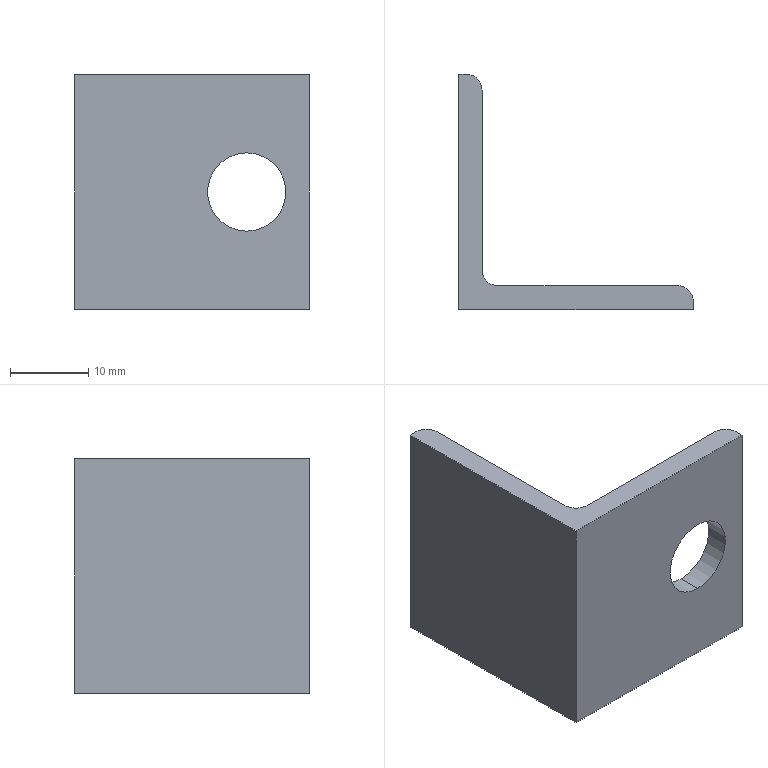Part | SolidWorks | features Extrusion 1, ICE 1 | 1 solid | 13 faces | box 30 x 30 x 30 mm | volume 4869 mm3 | plane 8 | cylinder 5 | commonest cylinder face diameters 4 x3 10 x2
STEP:
#1=CARTESIAN_POINT('',(22.,0.,10.));
#2=VERTEX_POINT('',#1);
#3=CARTESIAN_POINT('',(22.,0.,20.));
#4=VERTEX_POINT('',#3);
#5=CARTESIAN_POINT('',(22.,0.,15.));
#6=DIRECTION('',(0.,1.,0.));
#7=DIRECTION('',(0.,0.,1.));
#8=AXIS2_PLACEMENT_3D('',#5,#6,#7);
#9=CIRCLE('',#8,5.);
#10=EDGE_CURVE('',#2,#4,#9,.T.);
#11=ORIENTED_EDGE('',*,*,#10,.F.);
#12=CARTESIAN_POINT('',(22.,3.,10.));
#13=VERTEX_POINT('',#12);
#14=CARTESIAN_POINT('',(22.,0.,10.));
#15=DIRECTION('',(0.,1.,0.));
#16=VECTOR('',#15,1000.);
#17=LINE('',#14,#16);
#18=EDGE_CURVE('',#2,#13,#17,.T.);
#19=ORIENTED_EDGE('',*,*,#18,.T.);
#20=CARTESIAN_POINT('',(22.,3.,20.));
#21=VERTEX_POINT('',#20);
#22=CARTESIAN_POINT('',(22.,3.,15.));
#23=DIRECTION('',(0.,1.,0.));
#24=DIRECTION('',(0.,0.,1.));
#25=AXIS2_PLACEMENT_3D('',#22,#23,#24);
#26=CIRCLE('',#25,5.);
#27=EDGE_CURVE('',#13,#21,#26,.T.);
#28=ORIENTED_EDGE('',*,*,#27,.T.);
#29=CARTESIAN_POINT('',(22.,0.,20.));
#30=DIRECTION('',(0.,1.,0.));
#31=VECTOR('',#30,1000.);
#32=LINE('',#29,#31);
#33=EDGE_CURVE('',#4,#21,#32,.T.);
#34=ORIENTED_EDGE('',*,*,#33,.F.);
#35=EDGE_LOOP('',(#11,#19,#28,#34));
#36=FACE_OUTER_BOUND('',#35,.T.);
#37=CARTESIAN_POINT('',(22.,0.,15.));
#38=DIRECTION('',(0.,1.,0.));
#39=DIRECTION('',(0.,0.,1.));
#40=AXIS2_PLACEMENT_3D('',#37,#38,#39);
#41=CYLINDRICAL_SURFACE('',#40,5.);
#42=ADVANCED_FACE('',(#36),#41,.F.);
#43=CARTESIAN_POINT('',(22.,0.,15.));
#44=DIRECTION('',(0.,1.,0.));
#45=DIRECTION('',(0.,0.,1.));
#46=AXIS2_PLACEMENT_3D('',#43,#44,#45);
#47=CIRCLE('',#46,5.);
#48=EDGE_CURVE('',#4,#2,#47,.T.);
#49=ORIENTED_EDGE('',*,*,#48,.T.);
#50=ORIENTED_EDGE('',*,*,#10,.T.);
#51=EDGE_LOOP('',(#49,#50));
#52=FACE_BOUND('',#51,.T.);
#53=CARTESIAN_POINT('',(0.,0.,0.));
#54=VERTEX_POINT('',#53);
#55=CARTESIAN_POINT('',(30.,0.,0.));
#56=VERTEX_POINT('',#55);
#57=CARTESIAN_POINT('',(0.,0.,0.));
#58=DIRECTION('',(1.,0.,0.));
#59=VECTOR('',#58,1000.);
#60=LINE('',#57,#59);
#61=EDGE_CURVE('',#54,#56,#60,.T.);
#62=ORIENTED_EDGE('',*,*,#61,.T.);
#63=CARTESIAN_POINT('',(30.,0.,30.));
#64=VERTEX_POINT('',#63);
#65=CARTESIAN_POINT('',(30.,0.,30.));
#66=DIRECTION('',(0.,0.,-1.));
#67=VECTOR('',#66,1000.);
#68=LINE('',#65,#67);
#69=EDGE_CURVE('',#64,#56,#68,.T.);
#70=ORIENTED_EDGE('',*,*,#69,.F.);
#71=CARTESIAN_POINT('',(0.,0.,30.));
#72=VERTEX_POINT('',#71);
#73=CARTESIAN_POINT('',(0.,0.,30.));
#74=DIRECTION('',(1.,0.,0.));
#75=VECTOR('',#74,1000.);
#76=LINE('',#73,#75);
#77=EDGE_CURVE('',#72,#64,#76,.T.);
#78=ORIENTED_EDGE('',*,*,#77,.F.);
#79=CARTESIAN_POINT('',(0.,0.,30.));
#80=DIRECTION('',(0.,0.,-1.));
#81=VECTOR('',#80,1000.);
#82=LINE('',#79,#81);
#83=EDGE_CURVE('',#72,#54,#82,.T.);
#84=ORIENTED_EDGE('',*,*,#83,.T.);
#85=EDGE_LOOP('',(#62,#70,#78,#84));
#86=FACE_OUTER_BOUND('',#85,.T.);
#87=CARTESIAN_POINT('',(0.,0.,30.));
#88=DIRECTION('',(0.,1.,0.));
#89=DIRECTION('',(0.,0.,1.));
#90=AXIS2_PLACEMENT_3D('',#87,#88,#89);
#91=PLANE('',#90);
#92=ADVANCED_FACE('',(#52,#86),#91,.F.);
#93=CARTESIAN_POINT('',(30.,1.,0.));
#94=VERTEX_POINT('',#93);
#95=CARTESIAN_POINT('',(30.,1.,0.));
#96=DIRECTION('',(0.,1.,0.));
#97=VECTOR('',#96,1000.);
#98=LINE('',#95,#97);
#99=EDGE_CURVE('',#56,#94,#98,.T.);
#100=ORIENTED_EDGE('',*,*,#99,.T.);
#101=CARTESIAN_POINT('',(30.,1.,30.));
#102=VERTEX_POINT('',#101);
#103=CARTESIAN_POINT('',(30.,1.,30.));
#104=DIRECTION('',(0.,0.,-1.));
#105=VECTOR('',#104,1000.);
#106=LINE('',#103,#105);
#107=EDGE_CURVE('',#102,#94,#106,.T.);
#108=ORIENTED_EDGE('',*,*,#107,.F.);
#109=CARTESIAN_POINT('',(30.,1.,30.));
#110=DIRECTION('',(0.,1.,0.));
#111=VECTOR('',#110,1000.);
#112=LINE('',#109,#111);
#113=EDGE_CURVE('',#64,#102,#112,.T.);
#114=ORIENTED_EDGE('',*,*,#113,.F.);
#115=ORIENTED_EDGE('',*,*,#69,.T.);
#116=EDGE_LOOP('',(#100,#108,#114,#115));
#117=FACE_OUTER_BOUND('',#116,.T.);
#118=CARTESIAN_POINT('',(30.,1.,30.));
#119=DIRECTION('',(-1.,0.,0.));
#120=DIRECTION('',(0.,0.,1.));
#121=AXIS2_PLACEMENT_3D('',#118,#119,#120);
#122=PLANE('',#121);
#123=ADVANCED_FACE('',(#117),#122,.F.);
#124=CARTESIAN_POINT('',(28.,3.,0.));
#125=VERTEX_POINT('',#124);
#126=CARTESIAN_POINT('',(28.,1.,0.));
#127=DIRECTION('',(0.,0.,1.));
#128=DIRECTION('',(1.,0.,0.));
#129=AXIS2_PLACEMENT_3D('',#126,#127,#128);
#130=CIRCLE('',#129,2.);
#131=EDGE_CURVE('',#94,#125,#130,.T.);
#132=ORIENTED_EDGE('',*,*,#131,.T.);
#133=CARTESIAN_POINT('',(28.,3.,30.));
#134=VERTEX_POINT('',#133);
#135=CARTESIAN_POINT('',(28.,3.,30.));
#136=DIRECTION('',(0.,0.,-1.));
#137=VECTOR('',#136,1000.);
#138=LINE('',#135,#137);
#139=EDGE_CURVE('',#134,#125,#138,.T.);
#140=ORIENTED_EDGE('',*,*,#139,.F.);
#141=CARTESIAN_POINT('',(28.,1.,30.));
#142=DIRECTION('',(0.,0.,1.));
#143=DIRECTION('',(1.,0.,0.));
#144=AXIS2_PLACEMENT_3D('',#141,#142,#143);
#145=CIRCLE('',#144,2.);
#146=EDGE_CURVE('',#102,#134,#145,.T.);
#147=ORIENTED_EDGE('',*,*,#146,.F.);
#148=ORIENTED_EDGE('',*,*,#107,.T.);
#149=EDGE_LOOP('',(#132,#140,#147,#148));
#150=FACE_OUTER_BOUND('',#149,.T.);
#151=CARTESIAN_POINT('',(28.,1.,30.));
#152=DIRECTION('',(0.,0.,-1.));
#153=DIRECTION('',(-1.,0.,0.));
#154=AXIS2_PLACEMENT_3D('',#151,#152,#153);
#155=CYLINDRICAL_SURFACE('',#154,2.);
#156=ADVANCED_FACE('',(#150),#155,.T.);
#157=CARTESIAN_POINT('',(22.,3.,15.));
#158=DIRECTION('',(0.,1.,0.));
#159=DIRECTION('',(0.,0.,1.));
#160=AXIS2_PLACEMENT_3D('',#157,#158,#159);
#161=CIRCLE('',#160,5.);
#162=EDGE_CURVE('',#21,#13,#161,.T.);
#163=ORIENTED_EDGE('',*,*,#162,.F.);
#164=ORIENTED_EDGE('',*,*,#27,.F.);
#165=EDGE_LOOP('',(#163,#164));
#166=FACE_BOUND('',#165,.T.);
#167=CARTESIAN_POINT('',(5.,3.,0.));
#168=VERTEX_POINT('',#167);
#169=CARTESIAN_POINT('',(5.,3.,0.));
#170=DIRECTION('',(-1.,0.,0.));
#171=VECTOR('',#170,1000.);
#172=LINE('',#169,#171);
#173=EDGE_CURVE('',#125,#168,#172,.T.);
#174=ORIENTED_EDGE('',*,*,#173,.T.);
#175=CARTESIAN_POINT('',(5.,3.,30.));
#176=VERTEX_POINT('',#175);
#177=CARTESIAN_POINT('',(5.,3.,30.));
#178=DIRECTION('',(0.,0.,-1.));
#179=VECTOR('',#178,1000.);
#180=LINE('',#177,#179);
#181=EDGE_CURVE('',#176,#168,#180,.T.);
#182=ORIENTED_EDGE('',*,*,#181,.F.);
#183=CARTESIAN_POINT('',(5.,3.,30.));
#184=DIRECTION('',(-1.,0.,0.));
#185=VECTOR('',#184,1000.);
#186=LINE('',#183,#185);
#187=EDGE_CURVE('',#134,#176,#186,.T.);
#188=ORIENTED_EDGE('',*,*,#187,.F.);
#189=ORIENTED_EDGE('',*,*,#139,.T.);
#190=EDGE_LOOP('',(#174,#182,#188,#189));
#191=FACE_OUTER_BOUND('',#190,.T.);
#192=CARTESIAN_POINT('',(5.,3.,30.));
#193=DIRECTION('',(0.,-1.,0.));
#194=DIRECTION('',(0.,0.,-1.));
#195=AXIS2_PLACEMENT_3D('',#192,#193,#194);
#196=PLANE('',#195);
#197=ADVANCED_FACE('',(#166,#191),#196,.F.);
#198=CARTESIAN_POINT('',(3.,5.,0.));
#199=VERTEX_POINT('',#198);
#200=CARTESIAN_POINT('',(5.,5.,0.));
#201=DIRECTION('',(0.,0.,-1.));
#202=DIRECTION('',(-1.,0.,0.));
#203=AXIS2_PLACEMENT_3D('',#200,#201,#202);
#204=CIRCLE('',#203,2.);
#205=EDGE_CURVE('',#168,#199,#204,.T.);
#206=ORIENTED_EDGE('',*,*,#205,.T.);
#207=CARTESIAN_POINT('',(3.,5.,30.));
#208=VERTEX_POINT('',#207);
#209=CARTESIAN_POINT('',(3.,5.,30.));
#210=DIRECTION('',(0.,0.,-1.));
#211=VECTOR('',#210,1000.);
#212=LINE('',#209,#211);
#213=EDGE_CURVE('',#208,#199,#212,.T.);
#214=ORIENTED_EDGE('',*,*,#213,.F.);
#215=CARTESIAN_POINT('',(5.,5.,30.));
#216=DIRECTION('',(0.,0.,-1.));
#217=DIRECTION('',(-1.,0.,0.));
#218=AXIS2_PLACEMENT_3D('',#215,#216,#217);
#219=CIRCLE('',#218,2.);
#220=EDGE_CURVE('',#176,#208,#219,.T.);
#221=ORIENTED_EDGE('',*,*,#220,.F.);
#222=ORIENTED_EDGE('',*,*,#181,.T.);
#223=EDGE_LOOP('',(#206,#214,#221,#222));
#224=FACE_OUTER_BOUND('',#223,.T.);
#225=CARTESIAN_POINT('',(5.,5.,30.));
#226=DIRECTION('',(0.,0.,-1.));
#227=DIRECTION('',(-1.,0.,0.));
#228=AXIS2_PLACEMENT_3D('',#225,#226,#227);
#229=CYLINDRICAL_SURFACE('',#228,2.);
#230=ADVANCED_FACE('',(#224),#229,.F.);
#231=CARTESIAN_POINT('',(3.,28.,0.));
#232=VERTEX_POINT('',#231);
#233=CARTESIAN_POINT('',(3.,5.,0.));
#234=DIRECTION('',(0.,1.,0.));
#235=VECTOR('',#234,1000.);
#236=LINE('',#233,#235);
#237=EDGE_CURVE('',#199,#232,#236,.T.);
#238=ORIENTED_EDGE('',*,*,#237,.T.);
#239=CARTESIAN_POINT('',(3.,28.,30.));
#240=VERTEX_POINT('',#239);
#241=CARTESIAN_POINT('',(3.,28.,30.));
#242=DIRECTION('',(0.,0.,-1.));
#243=VECTOR('',#242,1000.);
#244=LINE('',#241,#243);
#245=EDGE_CURVE('',#240,#232,#244,.T.);
#246=ORIENTED_EDGE('',*,*,#245,.F.);
#247=CARTESIAN_POINT('',(3.,5.,30.));
#248=DIRECTION('',(0.,1.,0.));
#249=VECTOR('',#248,1000.);
#250=LINE('',#247,#249);
#251=EDGE_CURVE('',#208,#240,#250,.T.);
#252=ORIENTED_EDGE('',*,*,#251,.F.);
#253=ORIENTED_EDGE('',*,*,#213,.T.);
#254=EDGE_LOOP('',(#238,#246,#252,#253));
#255=FACE_OUTER_BOUND('',#254,.T.);
#256=CARTESIAN_POINT('',(3.,5.,30.));
#257=DIRECTION('',(-1.,0.,0.));
#258=DIRECTION('',(0.,0.,1.));
#259=AXIS2_PLACEMENT_3D('',#256,#257,#258);
#260=PLANE('',#259);
#261=ADVANCED_FACE('',(#255),#260,.F.);
#262=CARTESIAN_POINT('',(1.,30.,0.));
#263=VERTEX_POINT('',#262);
#264=CARTESIAN_POINT('',(1.,28.,0.));
#265=DIRECTION('',(0.,0.,1.));
#266=DIRECTION('',(1.,0.,0.));
#267=AXIS2_PLACEMENT_3D('',#264,#265,#266);
#268=CIRCLE('',#267,2.);
#269=EDGE_CURVE('',#232,#263,#268,.T.);
#270=ORIENTED_EDGE('',*,*,#269,.T.);
#271=CARTESIAN_POINT('',(1.,30.,30.));
#272=VERTEX_POINT('',#271);
#273=CARTESIAN_POINT('',(1.,30.,30.));
#274=DIRECTION('',(0.,0.,-1.));
#275=VECTOR('',#274,1000.);
#276=LINE('',#273,#275);
#277=EDGE_CURVE('',#272,#263,#276,.T.);
#278=ORIENTED_EDGE('',*,*,#277,.F.);
#279=CARTESIAN_POINT('',(1.,28.,30.));
#280=DIRECTION('',(0.,0.,1.));
#281=DIRECTION('',(1.,0.,0.));
#282=AXIS2_PLACEMENT_3D('',#279,#280,#281);
#283=CIRCLE('',#282,2.);
#284=EDGE_CURVE('',#240,#272,#283,.T.);
#285=ORIENTED_EDGE('',*,*,#284,.F.);
#286=ORIENTED_EDGE('',*,*,#245,.T.);
#287=EDGE_LOOP('',(#270,#278,#285,#286));
#288=FACE_OUTER_BOUND('',#287,.T.);
#289=CARTESIAN_POINT('',(1.,28.,30.));
#290=DIRECTION('',(0.,0.,-1.));
#291=DIRECTION('',(-1.,0.,0.));
#292=AXIS2_PLACEMENT_3D('',#289,#290,#291);
#293=CYLINDRICAL_SURFACE('',#292,2.);
#294=ADVANCED_FACE('',(#288),#293,.T.);
#295=CARTESIAN_POINT('',(0.,30.,0.));
#296=VERTEX_POINT('',#295);
#297=CARTESIAN_POINT('',(0.,30.,0.));
#298=DIRECTION('',(-1.,0.,0.));
#299=VECTOR('',#298,1000.);
#300=LINE('',#297,#299);
#301=EDGE_CURVE('',#263,#296,#300,.T.);
#302=ORIENTED_EDGE('',*,*,#301,.T.);
#303=CARTESIAN_POINT('',(0.,30.,30.));
#304=VERTEX_POINT('',#303);
#305=CARTESIAN_POINT('',(0.,30.,30.));
#306=DIRECTION('',(0.,0.,-1.));
#307=VECTOR('',#306,1000.);
#308=LINE('',#305,#307);
#309=EDGE_CURVE('',#304,#296,#308,.T.);
#310=ORIENTED_EDGE('',*,*,#309,.F.);
#311=CARTESIAN_POINT('',(0.,30.,30.));
#312=DIRECTION('',(-1.,0.,0.));
#313=VECTOR('',#312,1000.);
#314=LINE('',#311,#313);
#315=EDGE_CURVE('',#272,#304,#314,.T.);
#316=ORIENTED_EDGE('',*,*,#315,.F.);
#317=ORIENTED_EDGE('',*,*,#277,.T.);
#318=EDGE_LOOP('',(#302,#310,#316,#317));
#319=FACE_OUTER_BOUND('',#318,.T.);
#320=CARTESIAN_POINT('',(0.,30.,30.));
#321=DIRECTION('',(0.,-1.,0.));
#322=DIRECTION('',(0.,0.,-1.));
#323=AXIS2_PLACEMENT_3D('',#320,#321,#322);
#324=PLANE('',#323);
#325=ADVANCED_FACE('',(#319),#324,.F.);
#326=CARTESIAN_POINT('',(0.,0.,0.));
#327=DIRECTION('',(0.,-1.,0.));
#328=VECTOR('',#327,1000.);
#329=LINE('',#326,#328);
#330=EDGE_CURVE('',#296,#54,#329,.T.);
#331=ORIENTED_EDGE('',*,*,#330,.T.);
#332=ORIENTED_EDGE('',*,*,#83,.F.);
#333=CARTESIAN_POINT('',(0.,0.,30.));
#334=DIRECTION('',(0.,-1.,0.));
#335=VECTOR('',#334,1000.);
#336=LINE('',#333,#335);
#337=EDGE_CURVE('',#304,#72,#336,.T.);
#338=ORIENTED_EDGE('',*,*,#337,.F.);
#339=ORIENTED_EDGE('',*,*,#309,.T.);
#340=EDGE_LOOP('',(#331,#332,#338,#339));
#341=FACE_OUTER_BOUND('',#340,.T.);
#342=CARTESIAN_POINT('',(0.,0.,30.));
#343=DIRECTION('',(1.,0.,0.));
#344=DIRECTION('',(0.,0.,-1.));
#345=AXIS2_PLACEMENT_3D('',#342,#343,#344);
#346=PLANE('',#345);
#347=ADVANCED_FACE('',(#341),#346,.F.);
#348=ORIENTED_EDGE('',*,*,#77,.T.);
#349=ORIENTED_EDGE('',*,*,#113,.T.);
#350=ORIENTED_EDGE('',*,*,#146,.T.);
#351=ORIENTED_EDGE('',*,*,#187,.T.);
#352=ORIENTED_EDGE('',*,*,#220,.T.);
#353=ORIENTED_EDGE('',*,*,#251,.T.);
#354=ORIENTED_EDGE('',*,*,#284,.T.);
#355=ORIENTED_EDGE('',*,*,#315,.T.);
#356=ORIENTED_EDGE('',*,*,#337,.T.);
#357=EDGE_LOOP('',(#348,#349,#350,#351,#352,#353,#354,#355,#356));
#358=FACE_OUTER_BOUND('',#357,.T.);
#359=CARTESIAN_POINT('',(28.,1.,30.));
#360=DIRECTION('',(0.,0.,1.));
#361=DIRECTION('',(1.,0.,0.));
#362=AXIS2_PLACEMENT_3D('',#359,#360,#361);
#363=PLANE('',#362);
#364=ADVANCED_FACE('',(#358),#363,.T.);
#365=ORIENTED_EDGE('',*,*,#61,.F.);
#366=ORIENTED_EDGE('',*,*,#330,.F.);
#367=ORIENTED_EDGE('',*,*,#301,.F.);
#368=ORIENTED_EDGE('',*,*,#269,.F.);
#369=ORIENTED_EDGE('',*,*,#237,.F.);
#370=ORIENTED_EDGE('',*,*,#205,.F.);
#371=ORIENTED_EDGE('',*,*,#173,.F.);
#372=ORIENTED_EDGE('',*,*,#131,.F.);
#373=ORIENTED_EDGE('',*,*,#99,.F.);
#374=EDGE_LOOP('',(#365,#366,#367,#368,#369,#370,#371,#372,#373));
#375=FACE_OUTER_BOUND('',#374,.T.);
#376=CARTESIAN_POINT('',(28.,1.,0.));
#377=DIRECTION('',(0.,0.,1.));
#378=DIRECTION('',(1.,0.,0.));
#379=AXIS2_PLACEMENT_3D('',#376,#377,#378);
#380=PLANE('',#379);
#381=ADVANCED_FACE('',(#375),#380,.F.);
#382=ORIENTED_EDGE('',*,*,#18,.F.);
#383=ORIENTED_EDGE('',*,*,#48,.F.);
#384=ORIENTED_EDGE('',*,*,#33,.T.);
#385=ORIENTED_EDGE('',*,*,#162,.T.);
#386=EDGE_LOOP('',(#382,#383,#384,#385));
#387=FACE_OUTER_BOUND('',#386,.T.);
#388=CARTESIAN_POINT('',(22.,0.,15.));
#389=DIRECTION('',(0.,1.,0.));
#390=DIRECTION('',(0.,0.,1.));
#391=AXIS2_PLACEMENT_3D('',#388,#389,#390);
#392=CYLINDRICAL_SURFACE('',#391,5.);
#393=ADVANCED_FACE('',(#387),#392,.F.);
#394=CLOSED_SHELL('',(#42,#92,#123,#156,#197,#230,#261,#294,#325,#347,#364,#381,#393));
#395=MANIFOLD_SOLID_BREP('',#394);
#396=CARTESIAN_POINT('',(0.,0.,0.));
#397=DIRECTION('',(0.,0.,1.));
#398=DIRECTION('',(1.,0.,0.));
#399=AXIS2_PLACEMENT_3D('',#396,#397,#398);
#400=(LENGTH_UNIT()NAMED_UNIT(*)SI_UNIT(.MILLI.,.METRE.));
#401=UNCERTAINTY_MEASURE_WITH_UNIT(LENGTH_MEASURE(0.00001),#400,'','');
#402=(NAMED_UNIT(*)PLANE_ANGLE_UNIT()SI_UNIT($,.RADIAN.));
#403=(NAMED_UNIT(*)SI_UNIT($,.STERADIAN.)SOLID_ANGLE_UNIT());
#404=(GEOMETRIC_REPRESENTATION_CONTEXT(3)GLOBAL_UNCERTAINTY_ASSIGNED_CONTEXT((#401))GLOBAL_UNIT_ASSIGNED_CONTEXT((#400,#402,#403))REPRESENTATION_CONTEXT('',''));
#405=ADVANCED_BREP_SHAPE_REPRESENTATION('',(#395,#399),#404);